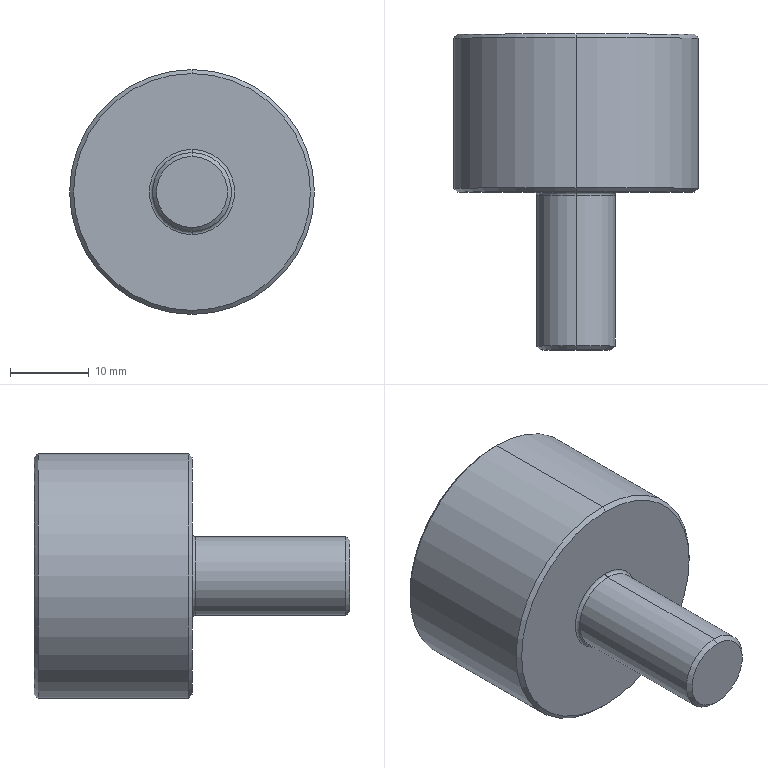Part | STEP file | OP10-133_seal rod camshaft | 1 solid | 25 faces | box 31 x 40 x 31 mm | volume 16299 mm3 | cylinder 10 | cone 8 | plane 5 | torus 2 | commonest cylinder face diameters 3.3 x2 6 x2 10 x2 11 x2 31 x2
STEP:
#1=CARTESIAN_POINT('',(0.,0.,0.));
#2=DIRECTION('',(0.,0.,1.));
#3=DIRECTION('',(1.,0.,0.));
#4=AXIS2_PLACEMENT_3D('',#1,#2,#3);
#5=CARTESIAN_POINT('',(0.,20.,5.4));
#6=VERTEX_POINT('',#5);
#7=CARTESIAN_POINT('',(0.,19.6,5.));
#8=VERTEX_POINT('',#7);
#9=CARTESIAN_POINT('',(0.,19.6,5.4));
#10=DIRECTION('',(-1.,0.,0.));
#11=DIRECTION('',(0.,0.,1.));
#12=AXIS2_PLACEMENT_3D('',#9,#10,#11);
#13=CIRCLE('',#12,0.4);
#14=CARTESIAN_POINT('',(0.,19.6,0.));
#15=DIRECTION('',(0.,1.,0.));
#16=DIRECTION('',(0.,0.,1.));
#17=AXIS2_PLACEMENT_3D('',#14,#15,#16);
#18=TOROIDAL_SURFACE('',#17,5.4,0.4);
#19=CARTESIAN_POINT('',(6.283,0.));
#20=DIRECTION('',(0.,1.));
#21=VECTOR('',#20,1.);
#22=LINE('',#19,#21);
#23=(GEOMETRIC_REPRESENTATION_CONTEXT(2)PARAMETRIC_REPRESENTATION_CONTEXT()REPRESENTATION_CONTEXT('',''));
#24=DEFINITIONAL_REPRESENTATION('',(#22),#23);
#25=PCURVE('',#18,#24);
#26=CARTESIAN_POINT('',(0.,19.6,0.));
#27=DIRECTION('',(0.,1.,0.));
#28=DIRECTION('',(0.,0.,1.));
#29=AXIS2_PLACEMENT_3D('',#26,#27,#28);
#30=TOROIDAL_SURFACE('',#29,5.4,0.4);
#31=CARTESIAN_POINT('',(0.,0.));
#32=DIRECTION('',(0.,1.));
#33=VECTOR('',#32,1.);
#34=LINE('',#31,#33);
#35=(GEOMETRIC_REPRESENTATION_CONTEXT(2)PARAMETRIC_REPRESENTATION_CONTEXT()REPRESENTATION_CONTEXT('',''));
#36=DEFINITIONAL_REPRESENTATION('',(#34),#35);
#37=PCURVE('',#30,#36);
#38=SURFACE_CURVE('',#13,(#25,#37),.PCURVE_S1.);
#39=EDGE_CURVE('',#6,#8,#38,.T.);
#40=ORIENTED_EDGE('',*,*,#39,.T.);
#41=CARTESIAN_POINT('',(0.,19.6,-5.));
#42=VERTEX_POINT('',#41);
#43=CARTESIAN_POINT('',(0.,19.6,0.));
#44=DIRECTION('',(0.,-1.,0.));
#45=DIRECTION('',(0.,0.,1.));
#46=AXIS2_PLACEMENT_3D('',#43,#44,#45);
#47=CIRCLE('',#46,5.);
#48=CARTESIAN_POINT('',(6.283,3.142));
#49=DIRECTION('',(-1.,0.));
#50=VECTOR('',#49,1.);
#51=LINE('',#48,#50);
#52=(GEOMETRIC_REPRESENTATION_CONTEXT(2)PARAMETRIC_REPRESENTATION_CONTEXT()REPRESENTATION_CONTEXT('',''));
#53=DEFINITIONAL_REPRESENTATION('',(#51),#52);
#54=PCURVE('',#18,#53);
#55=CARTESIAN_POINT('',(0.,20.,0.));
#56=DIRECTION('',(0.,-1.,0.));
#57=DIRECTION('',(0.,0.,-1.));
#58=AXIS2_PLACEMENT_3D('',#55,#56,#57);
#59=CYLINDRICAL_SURFACE('',#58,5.);
#60=CARTESIAN_POINT('',(3.142,0.4));
#61=DIRECTION('',(1.,0.));
#62=VECTOR('',#61,1.);
#63=LINE('',#60,#62);
#64=(GEOMETRIC_REPRESENTATION_CONTEXT(2)PARAMETRIC_REPRESENTATION_CONTEXT()REPRESENTATION_CONTEXT('',''));
#65=DEFINITIONAL_REPRESENTATION('',(#63),#64);
#66=PCURVE('',#59,#65);
#67=SURFACE_CURVE('',#47,(#54,#66),.PCURVE_S1.);
#68=EDGE_CURVE('',#8,#42,#67,.T.);
#69=ORIENTED_EDGE('',*,*,#68,.T.);
#70=CARTESIAN_POINT('',(0.,20.,-5.4));
#71=VERTEX_POINT('',#70);
#72=CARTESIAN_POINT('',(0.,19.6,-5.4));
#73=DIRECTION('',(1.,0.,0.));
#74=DIRECTION('',(0.,0.,-1.));
#75=AXIS2_PLACEMENT_3D('',#72,#73,#74);
#76=CIRCLE('',#75,0.4);
#77=CARTESIAN_POINT('',(3.142,0.));
#78=DIRECTION('',(0.,1.));
#79=VECTOR('',#78,1.);
#80=LINE('',#77,#79);
#81=(GEOMETRIC_REPRESENTATION_CONTEXT(2)PARAMETRIC_REPRESENTATION_CONTEXT()REPRESENTATION_CONTEXT('',''));
#82=DEFINITIONAL_REPRESENTATION('',(#80),#81);
#83=PCURVE('',#18,#82);
#84=CARTESIAN_POINT('',(3.142,0.));
#85=DIRECTION('',(0.,1.));
#86=VECTOR('',#85,1.);
#87=LINE('',#84,#86);
#88=(GEOMETRIC_REPRESENTATION_CONTEXT(2)PARAMETRIC_REPRESENTATION_CONTEXT()REPRESENTATION_CONTEXT('',''));
#89=DEFINITIONAL_REPRESENTATION('',(#87),#88);
#90=PCURVE('',#30,#89);
#91=SURFACE_CURVE('',#76,(#83,#90),.PCURVE_S1.);
#92=EDGE_CURVE('',#71,#42,#91,.T.);
#93=ORIENTED_EDGE('',*,*,#92,.F.);
#94=CARTESIAN_POINT('',(0.,20.,0.));
#95=DIRECTION('',(0.,1.,0.));
#96=DIRECTION('',(0.,0.,1.));
#97=AXIS2_PLACEMENT_3D('',#94,#95,#96);
#98=CIRCLE('',#97,5.4);
#99=CARTESIAN_POINT('',(0.,1.571));
#100=DIRECTION('',(1.,0.));
#101=VECTOR('',#100,1.);
#102=LINE('',#99,#101);
#103=(GEOMETRIC_REPRESENTATION_CONTEXT(2)PARAMETRIC_REPRESENTATION_CONTEXT()REPRESENTATION_CONTEXT('',''));
#104=DEFINITIONAL_REPRESENTATION('',(#102),#103);
#105=PCURVE('',#18,#104);
#106=CARTESIAN_POINT('',(0.,20.,0.));
#107=DIRECTION('',(0.,1.,0.));
#108=DIRECTION('',(0.,0.,1.));
#109=AXIS2_PLACEMENT_3D('',#106,#107,#108);
#110=PLANE('',#109);
#111=CARTESIAN_POINT('',(0.,0.));
#112=DIRECTION('',(1.,0.));
#113=AXIS2_PLACEMENT_2D('',#111,#112);
#114=CIRCLE('',#113,5.4);
#115=(GEOMETRIC_REPRESENTATION_CONTEXT(2)PARAMETRIC_REPRESENTATION_CONTEXT()REPRESENTATION_CONTEXT('',''));
#116=DEFINITIONAL_REPRESENTATION('',(#114),#115);
#117=PCURVE('',#110,#116);
#118=SURFACE_CURVE('',#98,(#105,#117),.PCURVE_S1.);
#119=EDGE_CURVE('',#71,#6,#118,.T.);
#120=ORIENTED_EDGE('',*,*,#119,.T.);
#121=EDGE_LOOP('',(#40,#69,#93,#120));
#122=FACE_BOUND('',#121,.F.);
#123=ADVANCED_FACE('',(#122),#18,.F.);
#124=CARTESIAN_POINT('',(0.,0.,-4.5));
#125=VERTEX_POINT('',#124);
#126=CARTESIAN_POINT('',(0.,0.,4.5));
#127=VERTEX_POINT('',#126);
#128=CARTESIAN_POINT('',(0.,0.,0.));
#129=DIRECTION('',(0.,-1.,0.));
#130=DIRECTION('',(0.,0.,1.));
#131=AXIS2_PLACEMENT_3D('',#128,#129,#130);
#132=CIRCLE('',#131,4.5);
#133=CARTESIAN_POINT('',(0.,0.5,0.));
#134=DIRECTION('',(0.,1.,0.));
#135=DIRECTION('',(0.,0.,1.));
#136=AXIS2_PLACEMENT_3D('',#133,#134,#135);
#137=CONICAL_SURFACE('',#136,5.,0.7854);
#138=CARTESIAN_POINT('',(6.283,-0.5));
#139=DIRECTION('',(-1.,0.));
#140=VECTOR('',#139,1.);
#141=LINE('',#138,#140);
#142=(GEOMETRIC_REPRESENTATION_CONTEXT(2)PARAMETRIC_REPRESENTATION_CONTEXT()REPRESENTATION_CONTEXT('',''));
#143=DEFINITIONAL_REPRESENTATION('',(#141),#142);
#144=PCURVE('',#137,#143);
#145=CARTESIAN_POINT('',(0.,0.,0.));
#146=DIRECTION('',(0.,1.,0.));
#147=DIRECTION('',(0.,0.,1.));
#148=AXIS2_PLACEMENT_3D('',#145,#146,#147);
#149=PLANE('',#148);
#150=CARTESIAN_POINT('',(4.5,0.));
#151=CARTESIAN_POINT('',(4.5,-7.794));
#152=CARTESIAN_POINT('',(-2.25,-3.897));
#153=CARTESIAN_POINT('',(-9.,0.));
#154=CARTESIAN_POINT('',(-2.25,3.897));
#155=CARTESIAN_POINT('',(4.5,7.794));
#156=CARTESIAN_POINT('',(4.5,0.));
#157=(BOUNDED_CURVE()B_SPLINE_CURVE(2,(#150,#151,#152,#153,#154,#155,#156),.UNSPECIFIED.,.T.,.F.)B_SPLINE_CURVE_WITH_KNOTS((1,2,2,2,2,1),(-2.094,0.,2.094,4.189,6.283,8.378),.UNSPECIFIED.)CURVE()GEOMETRIC_REPRESENTATION_ITEM()RATIONAL_B_SPLINE_CURVE((1.,0.5,1.,0.5,1.,0.5,1.))REPRESENTATION_ITEM(''));
#158=(GEOMETRIC_REPRESENTATION_CONTEXT(2)PARAMETRIC_REPRESENTATION_CONTEXT()REPRESENTATION_CONTEXT('',''));
#159=DEFINITIONAL_REPRESENTATION('',(#157),#158);
#160=PCURVE('',#149,#159);
#161=SURFACE_CURVE('',#132,(#144,#160),.PCURVE_S1.);
#162=EDGE_CURVE('',#125,#127,#161,.T.);
#163=ORIENTED_EDGE('',*,*,#162,.F.);
#164=CARTESIAN_POINT('',(0.,0.5,-5.));
#165=VERTEX_POINT('',#164);
#166=CARTESIAN_POINT('',(0.,0.5,-5.));
#167=DIRECTION('',(0.,0.7071,-0.7071));
#168=VECTOR('',#167,1.);
#169=LINE('',#166,#168);
#170=CARTESIAN_POINT('',(3.142,0.));
#171=DIRECTION('',(0.,1.));
#172=VECTOR('',#171,1.);
#173=LINE('',#170,#172);
#174=(GEOMETRIC_REPRESENTATION_CONTEXT(2)PARAMETRIC_REPRESENTATION_CONTEXT()REPRESENTATION_CONTEXT('',''));
#175=DEFINITIONAL_REPRESENTATION('',(#173),#174);
#176=PCURVE('',#137,#175);
#177=CARTESIAN_POINT('',(0.,0.5,0.));
#178=DIRECTION('',(0.,1.,0.));
#179=DIRECTION('',(0.,0.,1.));
#180=AXIS2_PLACEMENT_3D('',#177,#178,#179);
#181=CONICAL_SURFACE('',#180,5.,0.7854);
#182=CARTESIAN_POINT('',(3.142,0.));
#183=DIRECTION('',(0.,1.));
#184=VECTOR('',#183,1.);
#185=LINE('',#182,#184);
#186=(GEOMETRIC_REPRESENTATION_CONTEXT(2)PARAMETRIC_REPRESENTATION_CONTEXT()REPRESENTATION_CONTEXT('',''));
#187=DEFINITIONAL_REPRESENTATION('',(#185),#186);
#188=PCURVE('',#181,#187);
#189=SURFACE_CURVE('',#169,(#176,#188),.PCURVE_S1.);
#190=EDGE_CURVE('',#125,#165,#189,.T.);
#191=ORIENTED_EDGE('',*,*,#190,.T.);
#192=CARTESIAN_POINT('',(0.,0.5,5.));
#193=VERTEX_POINT('',#192);
#194=CARTESIAN_POINT('',(0.,0.5,0.));
#195=DIRECTION('',(0.,1.,0.));
#196=DIRECTION('',(0.,0.,1.));
#197=AXIS2_PLACEMENT_3D('',#194,#195,#196);
#198=CIRCLE('',#197,5.);
#199=CARTESIAN_POINT('',(0.,0.));
#200=DIRECTION('',(1.,0.));
#201=VECTOR('',#200,1.);
#202=LINE('',#199,#201);
#203=(GEOMETRIC_REPRESENTATION_CONTEXT(2)PARAMETRIC_REPRESENTATION_CONTEXT()REPRESENTATION_CONTEXT('',''));
#204=DEFINITIONAL_REPRESENTATION('',(#202),#203);
#205=PCURVE('',#137,#204);
#206=CARTESIAN_POINT('',(0.,20.,0.));
#207=DIRECTION('',(0.,-1.,0.));
#208=DIRECTION('',(0.,0.,-1.));
#209=AXIS2_PLACEMENT_3D('',#206,#207,#208);
#210=CYLINDRICAL_SURFACE('',#209,5.);
#211=CARTESIAN_POINT('',(3.142,19.5));
#212=DIRECTION('',(-1.,0.));
#213=VECTOR('',#212,1.);
#214=LINE('',#211,#213);
#215=(GEOMETRIC_REPRESENTATION_CONTEXT(2)PARAMETRIC_REPRESENTATION_CONTEXT()REPRESENTATION_CONTEXT('',''));
#216=DEFINITIONAL_REPRESENTATION('',(#214),#215);
#217=PCURVE('',#210,#216);
#218=SURFACE_CURVE('',#198,(#205,#217),.PCURVE_S1.);
#219=EDGE_CURVE('',#193,#165,#218,.T.);
#220=ORIENTED_EDGE('',*,*,#219,.F.);
#221=CARTESIAN_POINT('',(0.,0.5,5.));
#222=DIRECTION('',(0.,0.7071,0.7071));
#223=VECTOR('',#222,1.);
#224=LINE('',#221,#223);
#225=CARTESIAN_POINT('',(0.,0.));
#226=DIRECTION('',(0.,1.));
#227=VECTOR('',#226,1.);
#228=LINE('',#225,#227);
#229=(GEOMETRIC_REPRESENTATION_CONTEXT(2)PARAMETRIC_REPRESENTATION_CONTEXT()REPRESENTATION_CONTEXT('',''));
#230=DEFINITIONAL_REPRESENTATION('',(#228),#229);
#231=PCURVE('',#137,#230);
#232=CARTESIAN_POINT('',(6.283,0.));
#233=DIRECTION('',(0.,1.));
#234=VECTOR('',#233,1.);
#235=LINE('',#232,#234);
#236=(GEOMETRIC_REPRESENTATION_CONTEXT(2)PARAMETRIC_REPRESENTATION_CONTEXT()REPRESENTATION_CONTEXT('',''));
#237=DEFINITIONAL_REPRESENTATION('',(#235),#236);
#238=PCURVE('',#181,#237);
#239=SURFACE_CURVE('',#224,(#231,#238),.PCURVE_S1.);
#240=EDGE_CURVE('',#127,#193,#239,.T.);
#241=ORIENTED_EDGE('',*,*,#240,.F.);
#242=EDGE_LOOP('',(#163,#191,#220,#241));
#243=FACE_BOUND('',#242,.T.);
#244=ADVANCED_FACE('',(#243),#137,.T.);
#245=CARTESIAN_POINT('',(0.,40.,15.));
#246=VERTEX_POINT('',#245);
#247=CARTESIAN_POINT('',(0.,40.,-15.));
#248=VERTEX_POINT('',#247);
#249=CARTESIAN_POINT('',(0.,40.,0.));
#250=DIRECTION('',(0.,1.,0.));
#251=DIRECTION('',(0.,0.,1.));
#252=AXIS2_PLACEMENT_3D('',#249,#250,#251);
#253=CIRCLE('',#252,15.);
#254=CARTESIAN_POINT('',(0.,40.,0.));
#255=DIRECTION('',(0.,-1.,0.));
#256=DIRECTION('',(0.,0.,-1.));
#257=AXIS2_PLACEMENT_3D('',#254,#255,#256);
#258=CONICAL_SURFACE('',#257,15.,0.7854);
#259=CARTESIAN_POINT('',(3.142,0.));
#260=DIRECTION('',(-1.,0.));
#261=VECTOR('',#260,1.);
#262=LINE('',#259,#261);
#263=(GEOMETRIC_REPRESENTATION_CONTEXT(2)PARAMETRIC_REPRESENTATION_CONTEXT()REPRESENTATION_CONTEXT('',''));
#264=DEFINITIONAL_REPRESENTATION('',(#262),#263);
#265=PCURVE('',#258,#264);
#266=CARTESIAN_POINT('',(0.,40.,0.));
#267=DIRECTION('',(0.,1.,0.));
#268=DIRECTION('',(0.,0.,1.));
#269=AXIS2_PLACEMENT_3D('',#266,#267,#268);
#270=PLANE('',#269);
#271=CARTESIAN_POINT('',(0.,0.));
#272=DIRECTION('',(1.,0.));
#273=AXIS2_PLACEMENT_2D('',#271,#272);
#274=CIRCLE('',#273,15.);
#275=(GEOMETRIC_REPRESENTATION_CONTEXT(2)PARAMETRIC_REPRESENTATION_CONTEXT()REPRESENTATION_CONTEXT('',''));
#276=DEFINITIONAL_REPRESENTATION('',(#274),#275);
#277=PCURVE('',#270,#276);
#278=SURFACE_CURVE('',#253,(#265,#277),.PCURVE_S1.);
#279=EDGE_CURVE('',#246,#248,#278,.T.);
#280=ORIENTED_EDGE('',*,*,#279,.F.);
#281=CARTESIAN_POINT('',(0.,39.5,15.5));
#282=VERTEX_POINT('',#281);
#283=CARTESIAN_POINT('',(0.,40.,15.));
#284=DIRECTION('',(0.,-0.7071,0.7071));
#285=VECTOR('',#284,1.);
#286=LINE('',#283,#285);
#287=CARTESIAN_POINT('',(3.142,0.));
#288=DIRECTION('',(0.,1.));
#289=VECTOR('',#288,1.);
#290=LINE('',#287,#289);
#291=(GEOMETRIC_REPRESENTATION_CONTEXT(2)PARAMETRIC_REPRESENTATION_CONTEXT()REPRESENTATION_CONTEXT('',''));
#292=DEFINITIONAL_REPRESENTATION('',(#290),#291);
#293=PCURVE('',#258,#292);
#294=CARTESIAN_POINT('',(0.,40.,0.));
#295=DIRECTION('',(0.,-1.,0.));
#296=DIRECTION('',(0.,0.,-1.));
#297=AXIS2_PLACEMENT_3D('',#294,#295,#296);
#298=CONICAL_SURFACE('',#297,15.,0.7854);
#299=CARTESIAN_POINT('',(3.142,0.));
#300=DIRECTION('',(0.,1.));
#301=VECTOR('',#300,1.);
#302=LINE('',#299,#301);
#303=(GEOMETRIC_REPRESENTATION_CONTEXT(2)PARAMETRIC_REPRESENTATION_CONTEXT()REPRESENTATION_CONTEXT('',''));
#304=DEFINITIONAL_REPRESENTATION('',(#302),#303);
#305=PCURVE('',#298,#304);
#306=SURFACE_CURVE('',#286,(#293,#305),.PCURVE_S1.);
#307=EDGE_CURVE('',#246,#282,#306,.T.);
#308=ORIENTED_EDGE('',*,*,#307,.T.);
#309=CARTESIAN_POINT('',(0.,39.5,-15.5));
#310=VERTEX_POINT('',#309);
#311=CARTESIAN_POINT('',(0.,39.5,0.));
#312=DIRECTION('',(0.,-1.,0.));
#313=DIRECTION('',(0.,0.,1.));
#314=AXIS2_PLACEMENT_3D('',#311,#312,#313);
#315=CIRCLE('',#314,15.5);
#316=CARTESIAN_POINT('',(-3.142,0.5));
#317=DIRECTION('',(1.,0.));
#318=VECTOR('',#317,1.);
#319=LINE('',#316,#318);
#320=(GEOMETRIC_REPRESENTATION_CONTEXT(2)PARAMETRIC_REPRESENTATION_CONTEXT()REPRESENTATION_CONTEXT('',''));
#321=DEFINITIONAL_REPRESENTATION('',(#319),#320);
#322=PCURVE('',#258,#321);
#323=CARTESIAN_POINT('',(0.,40.,0.));
#324=DIRECTION('',(0.,-1.,0.));
#325=DIRECTION('',(0.,0.,-1.));
#326=AXIS2_PLACEMENT_3D('',#323,#324,#325);
#327=CYLINDRICAL_SURFACE('',#326,15.5);
#328=CARTESIAN_POINT('',(-3.142,0.5));
#329=DIRECTION('',(1.,0.));
#330=VECTOR('',#329,1.);
#331=LINE('',#328,#330);
#332=(GEOMETRIC_REPRESENTATION_CONTEXT(2)PARAMETRIC_REPRESENTATION_CONTEXT()REPRESENTATION_CONTEXT('',''));
#333=DEFINITIONAL_REPRESENTATION('',(#331),#332);
#334=PCURVE('',#327,#333);
#335=SURFACE_CURVE('',#315,(#322,#334),.PCURVE_S1.);
#336=EDGE_CURVE('',#310,#282,#335,.T.);
#337=ORIENTED_EDGE('',*,*,#336,.F.);
#338=CARTESIAN_POINT('',(0.,40.,-15.));
#339=DIRECTION('',(0.,-0.7071,-0.7071));
#340=VECTOR('',#339,1.);
#341=LINE('',#338,#340);
#342=CARTESIAN_POINT('',(0.,0.));
#343=DIRECTION('',(0.,1.));
#344=VECTOR('',#343,1.);
#345=LINE('',#342,#344);
#346=(GEOMETRIC_REPRESENTATION_CONTEXT(2)PARAMETRIC_REPRESENTATION_CONTEXT()REPRESENTATION_CONTEXT('',''));
#347=DEFINITIONAL_REPRESENTATION('',(#345),#346);
#348=PCURVE('',#258,#347);
#349=CARTESIAN_POINT('',(6.283,0.));
#350=DIRECTION('',(0.,1.));
#351=VECTOR('',#350,1.);
#352=LINE('',#349,#351);
#353=(GEOMETRIC_REPRESENTATION_CONTEXT(2)PARAMETRIC_REPRESENTATION_CONTEXT()REPRESENTATION_CONTEXT('',''));
#354=DEFINITIONAL_REPRESENTATION('',(#352),#353);
#355=PCURVE('',#298,#354);
#356=SURFACE_CURVE('',#341,(#348,#355),.PCURVE_S1.);
#357=EDGE_CURVE('',#248,#310,#356,.T.);
#358=ORIENTED_EDGE('',*,*,#357,.F.);
#359=EDGE_LOOP('',(#280,#308,#337,#358));
#360=FACE_BOUND('',#359,.T.);
#361=ADVANCED_FACE('',(#360),#258,.T.);
#362=CARTESIAN_POINT('',(0.,20.,-15.));
#363=VERTEX_POINT('',#362);
#364=CARTESIAN_POINT('',(0.,20.,15.));
#365=VERTEX_POINT('',#364);
#366=CARTESIAN_POINT('',(0.,20.,0.));
#367=DIRECTION('',(0.,-1.,0.));
#368=DIRECTION('',(0.,0.,1.));
#369=AXIS2_PLACEMENT_3D('',#366,#367,#368);
#370=CIRCLE('',#369,15.);
#371=CARTESIAN_POINT('',(0.,20.5,0.));
#372=DIRECTION('',(0.,1.,0.));
#373=DIRECTION('',(0.,0.,1.));
#374=AXIS2_PLACEMENT_3D('',#371,#372,#373);
#375=CONICAL_SURFACE('',#374,15.5,0.7854);
#376=CARTESIAN_POINT('',(6.283,-0.5));
#377=DIRECTION('',(-1.,0.));
#378=VECTOR('',#377,1.);
#379=LINE('',#376,#378);
#380=(GEOMETRIC_REPRESENTATION_CONTEXT(2)PARAMETRIC_REPRESENTATION_CONTEXT()REPRESENTATION_CONTEXT('',''));
#381=DEFINITIONAL_REPRESENTATION('',(#379),#380);
#382=PCURVE('',#375,#381);
#383=CARTESIAN_POINT('',(15.,0.));
#384=CARTESIAN_POINT('',(15.,-25.981));
#385=CARTESIAN_POINT('',(-7.5,-12.99));
#386=CARTESIAN_POINT('',(-30.,0.));
#387=CARTESIAN_POINT('',(-7.5,12.99));
#388=CARTESIAN_POINT('',(15.,25.981));
#389=CARTESIAN_POINT('',(15.,0.));
#390=(BOUNDED_CURVE()B_SPLINE_CURVE(2,(#383,#384,#385,#386,#387,#388,#389),.UNSPECIFIED.,.T.,.F.)B_SPLINE_CURVE_WITH_KNOTS((1,2,2,2,2,1),(-2.094,0.,2.094,4.189,6.283,8.378),.UNSPECIFIED.)CURVE()GEOMETRIC_REPRESENTATION_ITEM()RATIONAL_B_SPLINE_CURVE((1.,0.5,1.,0.5,1.,0.5,1.))REPRESENTATION_ITEM(''));
#391=(GEOMETRIC_REPRESENTATION_CONTEXT(2)PARAMETRIC_REPRESENTATION_CONTEXT()REPRESENTATION_CONTEXT('',''));
#392=DEFINITIONAL_REPRESENTATION('',(#390),#391);
#393=PCURVE('',#110,#392);
#394=SURFACE_CURVE('',#370,(#382,#393),.PCURVE_S1.);
#395=EDGE_CURVE('',#363,#365,#394,.T.);
#396=ORIENTED_EDGE('',*,*,#395,.F.);
#397=CARTESIAN_POINT('',(0.,20.5,-15.5));
#398=VERTEX_POINT('',#397);
#399=CARTESIAN_POINT('',(0.,20.5,-15.5));
#400=DIRECTION('',(0.,0.7071,-0.7071));
#401=VECTOR('',#400,1.);
#402=LINE('',#399,#401);
#403=CARTESIAN_POINT('',(3.142,0.));
#404=DIRECTION('',(0.,1.));
#405=VECTOR('',#404,1.);
#406=LINE('',#403,#405);
#407=(GEOMETRIC_REPRESENTATION_CONTEXT(2)PARAMETRIC_REPRESENTATION_CONTEXT()REPRESENTATION_CONTEXT('',''));
#408=DEFINITIONAL_REPRESENTATION('',(#406),#407);
#409=PCURVE('',#375,#408);
#410=CARTESIAN_POINT('',(0.,20.5,0.));
#411=DIRECTION('',(0.,1.,0.));
#412=DIRECTION('',(0.,0.,1.));
#413=AXIS2_PLACEMENT_3D('',#410,#411,#412);
#414=CONICAL_SURFACE('',#413,15.5,0.7854);
#415=CARTESIAN_POINT('',(3.142,0.));
#416=DIRECTION('',(0.,1.));
#417=VECTOR('',#416,1.);
#418=LINE('',#415,#417);
#419=(GEOMETRIC_REPRESENTATION_CONTEXT(2)PARAMETRIC_REPRESENTATION_CONTEXT()REPRESENTATION_CONTEXT('',''));
#420=DEFINITIONAL_REPRESENTATION('',(#418),#419);
#421=PCURVE('',#414,#420);
#422=SURFACE_CURVE('',#402,(#409,#421),.PCURVE_S1.);
#423=EDGE_CURVE('',#363,#398,#422,.T.);
#424=ORIENTED_EDGE('',*,*,#423,.T.);
#425=CARTESIAN_POINT('',(0.,20.5,15.5));
#426=VERTEX_POINT('',#425);
#427=CARTESIAN_POINT('',(0.,20.5,0.));
#428=DIRECTION('',(0.,1.,0.));
#429=DIRECTION('',(0.,0.,1.));
#430=AXIS2_PLACEMENT_3D('',#427,#428,#429);
#431=CIRCLE('',#430,15.5);
#432=CARTESIAN_POINT('',(0.,0.));
#433=DIRECTION('',(1.,0.));
#434=VECTOR('',#433,1.);
#435=LINE('',#432,#434);
#436=(GEOMETRIC_REPRESENTATION_CONTEXT(2)PARAMETRIC_REPRESENTATION_CONTEXT()REPRESENTATION_CONTEXT('',''));
#437=DEFINITIONAL_REPRESENTATION('',(#435),#436);
#438=PCURVE('',#375,#437);
#439=CARTESIAN_POINT('',(3.142,19.5));
#440=DIRECTION('',(-1.,0.));
#441=VECTOR('',#440,1.);
#442=LINE('',#439,#441);
#443=(GEOMETRIC_REPRESENTATION_CONTEXT(2)PARAMETRIC_REPRESENTATION_CONTEXT()REPRESENTATION_CONTEXT('',''));
#444=DEFINITIONAL_REPRESENTATION('',(#442),#443);
#445=PCURVE('',#327,#444);
#446=SURFACE_CURVE('',#431,(#438,#445),.PCURVE_S1.);
#447=EDGE_CURVE('',#426,#398,#446,.T.);
#448=ORIENTED_EDGE('',*,*,#447,.F.);
#449=CARTESIAN_POINT('',(0.,20.5,15.5));
#450=DIRECTION('',(0.,0.7071,0.7071));
#451=VECTOR('',#450,1.);
#452=LINE('',#449,#451);
#453=CARTESIAN_POINT('',(0.,0.));
#454=DIRECTION('',(0.,1.));
#455=VECTOR('',#454,1.);
#456=LINE('',#453,#455);
#457=(GEOMETRIC_REPRESENTATION_CONTEXT(2)PARAMETRIC_REPRESENTATION_CONTEXT()REPRESENTATION_CONTEXT('',''));
#458=DEFINITIONAL_REPRESENTATION('',(#456),#457);
#459=PCURVE('',#375,#458);
#460=CARTESIAN_POINT('',(6.283,0.));
#461=DIRECTION('',(0.,1.));
#462=VECTOR('',#461,1.);
#463=LINE('',#460,#462);
#464=(GEOMETRIC_REPRESENTATION_CONTEXT(2)PARAMETRIC_REPRESENTATION_CONTEXT()REPRESENTATION_CONTEXT('',''));
#465=DEFINITIONAL_REPRESENTATION('',(#463),#464);
#466=PCURVE('',#414,#465);
#467=SURFACE_CURVE('',#452,(#459,#466),.PCURVE_S1.);
#468=EDGE_CURVE('',#365,#426,#467,.T.);
#469=ORIENTED_EDGE('',*,*,#468,.F.);
#470=EDGE_LOOP('',(#396,#424,#448,#469));
#471=FACE_BOUND('',#470,.T.);
#472=ADVANCED_FACE('',(#471),#375,.T.);
#473=CARTESIAN_POINT('',(0.,23.,1.65));
#474=VERTEX_POINT('',#473);
#475=CARTESIAN_POINT('',(0.,35.,1.65));
#476=VERTEX_POINT('',#475);
#477=CARTESIAN_POINT('',(0.,35.,1.65));
#478=DIRECTION('',(0.,1.,0.));
#479=VECTOR('',#478,1.);
#480=LINE('',#477,#479);
#481=CARTESIAN_POINT('',(0.,35.,0.));
#482=DIRECTION('',(0.,1.,0.));
#483=DIRECTION('',(0.,0.,1.));
#484=AXIS2_PLACEMENT_3D('',#481,#482,#483);
#485=CYLINDRICAL_SURFACE('',#484,1.65);
#486=CARTESIAN_POINT('',(6.283,0.));
#487=DIRECTION('',(0.,1.));
#488=VECTOR('',#487,1.);
#489=LINE('',#486,#488);
#490=(GEOMETRIC_REPRESENTATION_CONTEXT(2)PARAMETRIC_REPRESENTATION_CONTEXT()REPRESENTATION_CONTEXT('',''));
#491=DEFINITIONAL_REPRESENTATION('',(#489),#490);
#492=PCURVE('',#485,#491);
#493=CARTESIAN_POINT('',(0.,35.,0.));
#494=DIRECTION('',(0.,1.,0.));
#495=DIRECTION('',(0.,0.,1.));
#496=AXIS2_PLACEMENT_3D('',#493,#494,#495);
#497=CYLINDRICAL_SURFACE('',#496,1.65);
#498=CARTESIAN_POINT('',(0.,0.));
#499=DIRECTION('',(0.,1.));
#500=VECTOR('',#499,1.);
#501=LINE('',#498,#500);
#502=(GEOMETRIC_REPRESENTATION_CONTEXT(2)PARAMETRIC_REPRESENTATION_CONTEXT()REPRESENTATION_CONTEXT('',''));
#503=DEFINITIONAL_REPRESENTATION('',(#501),#502);
#504=PCURVE('',#497,#503);
#505=SURFACE_CURVE('',#480,(#492,#504),.PCURVE_S1.);
#506=EDGE_CURVE('',#474,#476,#505,.T.);
#507=ORIENTED_EDGE('',*,*,#506,.T.);
#508=CARTESIAN_POINT('',(0.,35.,-1.65));
#509=VERTEX_POINT('',#508);
#510=CARTESIAN_POINT('',(0.,35.,0.));
#511=DIRECTION('',(0.,1.,0.));
#512=DIRECTION('',(0.,0.,1.));
#513=AXIS2_PLACEMENT_3D('',#510,#511,#512);
#514=CIRCLE('',#513,1.65);
#515=CARTESIAN_POINT('',(0.,0.));
#516=DIRECTION('',(1.,0.));
#517=VECTOR('',#516,1.);
#518=LINE('',#515,#517);
#519=(GEOMETRIC_REPRESENTATION_CONTEXT(2)PARAMETRIC_REPRESENTATION_CONTEXT()REPRESENTATION_CONTEXT('',''));
#520=DEFINITIONAL_REPRESENTATION('',(#518),#519);
#521=PCURVE('',#485,#520);
#522=CARTESIAN_POINT('',(0.,35.,0.));
#523=DIRECTION('',(0.,1.,0.));
#524=DIRECTION('',(0.,0.,1.));
#525=AXIS2_PLACEMENT_3D('',#522,#523,#524);
#526=PLANE('',#525);
#527=CARTESIAN_POINT('',(0.,0.));
#528=DIRECTION('',(1.,0.));
#529=AXIS2_PLACEMENT_2D('',#527,#528);
#530=CIRCLE('',#529,1.65);
#531=(GEOMETRIC_REPRESENTATION_CONTEXT(2)PARAMETRIC_REPRESENTATION_CONTEXT()REPRESENTATION_CONTEXT('',''));
#532=DEFINITIONAL_REPRESENTATION('',(#530),#531);
#533=PCURVE('',#526,#532);
#534=SURFACE_CURVE('',#514,(#521,#533),.PCURVE_S1.);
#535=EDGE_CURVE('',#509,#476,#534,.T.);
#536=ORIENTED_EDGE('',*,*,#535,.F.);
#537=CARTESIAN_POINT('',(0.,23.,-1.65));
#538=VERTEX_POINT('',#537);
#539=CARTESIAN_POINT('',(0.,35.,-1.65));
#540=DIRECTION('',(0.,1.,0.));
#541=VECTOR('',#540,1.);
#542=LINE('',#539,#541);
#543=CARTESIAN_POINT('',(3.142,0.));
#544=DIRECTION('',(0.,1.));
#545=VECTOR('',#544,1.);
#546=LINE('',#543,#545);
#547=(GEOMETRIC_REPRESENTATION_CONTEXT(2)PARAMETRIC_REPRESENTATION_CONTEXT()REPRESENTATION_CONTEXT('',''));
#548=DEFINITIONAL_REPRESENTATION('',(#546),#547);
#549=PCURVE('',#485,#548);
#550=CARTESIAN_POINT('',(3.142,0.));
#551=DIRECTION('',(0.,1.));
#552=VECTOR('',#551,1.);
#553=LINE('',#550,#552);
#554=(GEOMETRIC_REPRESENTATION_CONTEXT(2)PARAMETRIC_REPRESENTATION_CONTEXT()REPRESENTATION_CONTEXT('',''));
#555=DEFINITIONAL_REPRESENTATION('',(#553),#554);
#556=PCURVE('',#497,#555);
#557=SURFACE_CURVE('',#542,(#549,#556),.PCURVE_S1.);
#558=EDGE_CURVE('',#538,#509,#557,.T.);
#559=ORIENTED_EDGE('',*,*,#558,.F.);
#560=CARTESIAN_POINT('',(0.,23.,0.));
#561=DIRECTION('',(0.,1.,0.));
#562=DIRECTION('',(0.,0.,1.));
#563=AXIS2_PLACEMENT_3D('',#560,#561,#562);
#564=CIRCLE('',#563,1.65);
#565=CARTESIAN_POINT('',(0.,-12.));
#566=DIRECTION('',(1.,0.));
#567=VECTOR('',#566,1.);
#568=LINE('',#565,#567);
#569=(GEOMETRIC_REPRESENTATION_CONTEXT(2)PARAMETRIC_REPRESENTATION_CONTEXT()REPRESENTATION_CONTEXT('',''));
#570=DEFINITIONAL_REPRESENTATION('',(#568),#569);
#571=PCURVE('',#485,#570);
#572=CARTESIAN_POINT('',(0.,23.,0.));
#573=DIRECTION('',(0.,1.,0.));
#574=DIRECTION('',(0.,0.,1.));
#575=AXIS2_PLACEMENT_3D('',#572,#573,#574);
#576=CONICAL_SURFACE('',#575,1.65,1.03);
#577=CARTESIAN_POINT('',(0.,0.));
#578=DIRECTION('',(1.,0.));
#579=VECTOR('',#578,1.);
#580=LINE('',#577,#579);
#581=(GEOMETRIC_REPRESENTATION_CONTEXT(2)PARAMETRIC_REPRESENTATION_CONTEXT()REPRESENTATION_CONTEXT('',''));
#582=DEFINITIONAL_REPRESENTATION('',(#580),#581);
#583=PCURVE('',#576,#582);
#584=SURFACE_CURVE('',#564,(#571,#583),.PCURVE_S1.);
#585=EDGE_CURVE('',#538,#474,#584,.T.);
#586=ORIENTED_EDGE('',*,*,#585,.T.);
#587=EDGE_LOOP('',(#507,#536,#559,#586));
#588=FACE_BOUND('',#587,.F.);
#589=ADVANCED_FACE('',(#588),#485,.F.);
#590=ORIENTED_EDGE('',*,*,#585,.F.);
#591=CARTESIAN_POINT('',(0.,22.009,0.));
#592=VERTEX_POINT('',#591);
#593=CARTESIAN_POINT('',(0.,23.,-1.65));
#594=DIRECTION('',(0.,0.515,-0.8572));
#595=VECTOR('',#594,1.);
#596=LINE('',#593,#595);
#597=CARTESIAN_POINT('',(3.142,0.));
#598=DIRECTION('',(0.,1.));
#599=VECTOR('',#598,1.);
#600=LINE('',#597,#599);
#601=(GEOMETRIC_REPRESENTATION_CONTEXT(2)PARAMETRIC_REPRESENTATION_CONTEXT()REPRESENTATION_CONTEXT('',''));
#602=DEFINITIONAL_REPRESENTATION('',(#600),#601);
#603=PCURVE('',#576,#602);
#604=CARTESIAN_POINT('',(0.,23.,0.));
#605=DIRECTION('',(0.,1.,0.));
#606=DIRECTION('',(0.,0.,1.));
#607=AXIS2_PLACEMENT_3D('',#604,#605,#606);
#608=CONICAL_SURFACE('',#607,1.65,1.03);
#609=CARTESIAN_POINT('',(3.142,0.));
#610=DIRECTION('',(0.,1.));
#611=VECTOR('',#610,1.);
#612=LINE('',#609,#611);
#613=(GEOMETRIC_REPRESENTATION_CONTEXT(2)PARAMETRIC_REPRESENTATION_CONTEXT()REPRESENTATION_CONTEXT('',''));
#614=DEFINITIONAL_REPRESENTATION('',(#612),#613);
#615=PCURVE('',#608,#614);
#616=SURFACE_CURVE('',#596,(#603,#615),.PCURVE_S1.);
#617=EDGE_CURVE('',#592,#538,#616,.T.);
#618=ORIENTED_EDGE('',*,*,#617,.F.);
#619=CARTESIAN_POINT('',(0.,23.,1.65));
#620=DIRECTION('',(0.,0.515,0.8572));
#621=VECTOR('',#620,1.);
#622=LINE('',#619,#621);
#623=CARTESIAN_POINT('',(6.283,0.));
#624=DIRECTION('',(0.,1.));
#625=VECTOR('',#624,1.);
#626=LINE('',#623,#625);
#627=(GEOMETRIC_REPRESENTATION_CONTEXT(2)PARAMETRIC_REPRESENTATION_CONTEXT()REPRESENTATION_CONTEXT('',''));
#628=DEFINITIONAL_REPRESENTATION('',(#626),#627);
#629=PCURVE('',#576,#628);
#630=CARTESIAN_POINT('',(0.,0.));
#631=DIRECTION('',(0.,1.));
#632=VECTOR('',#631,1.);
#633=LINE('',#630,#632);
#634=(GEOMETRIC_REPRESENTATION_CONTEXT(2)PARAMETRIC_REPRESENTATION_CONTEXT()REPRESENTATION_CONTEXT('',''));
#635=DEFINITIONAL_REPRESENTATION('',(#633),#634);
#636=PCURVE('',#608,#635);
#637=SURFACE_CURVE('',#622,(#629,#636),.PCURVE_S1.);
#638=EDGE_CURVE('',#592,#474,#637,.T.);
#639=ORIENTED_EDGE('',*,*,#638,.T.);
#640=EDGE_LOOP('',(#590,#618,#639));
#641=FACE_BOUND('',#640,.F.);
#642=ADVANCED_FACE('',(#641),#576,.F.);
#643=CARTESIAN_POINT('',(0.,35.,3.));
#644=VERTEX_POINT('',#643);
#645=CARTESIAN_POINT('',(0.,38.6,3.));
#646=VERTEX_POINT('',#645);
#647=CARTESIAN_POINT('',(0.,35.,3.));
#648=DIRECTION('',(0.,1.,0.));
#649=VECTOR('',#648,1.);
#650=LINE('',#647,#649);
#651=CARTESIAN_POINT('',(0.,35.,0.));
#652=DIRECTION('',(0.,1.,0.));
#653=DIRECTION('',(0.,0.,1.));
#654=AXIS2_PLACEMENT_3D('',#651,#652,#653);
#655=CYLINDRICAL_SURFACE('',#654,3.);
#656=CARTESIAN_POINT('',(6.283,0.));
#657=DIRECTION('',(0.,1.));
#658=VECTOR('',#657,1.);
#659=LINE('',#656,#658);
#660=(GEOMETRIC_REPRESENTATION_CONTEXT(2)PARAMETRIC_REPRESENTATION_CONTEXT()REPRESENTATION_CONTEXT('',''));
#661=DEFINITIONAL_REPRESENTATION('',(#659),#660);
#662=PCURVE('',#655,#661);
#663=CARTESIAN_POINT('',(0.,35.,0.));
#664=DIRECTION('',(0.,1.,0.));
#665=DIRECTION('',(0.,0.,1.));
#666=AXIS2_PLACEMENT_3D('',#663,#664,#665);
#667=CYLINDRICAL_SURFACE('',#666,3.);
#668=CARTESIAN_POINT('',(0.,0.));
#669=DIRECTION('',(0.,1.));
#670=VECTOR('',#669,1.);
#671=LINE('',#668,#670);
#672=(GEOMETRIC_REPRESENTATION_CONTEXT(2)PARAMETRIC_REPRESENTATION_CONTEXT()REPRESENTATION_CONTEXT('',''));
#673=DEFINITIONAL_REPRESENTATION('',(#671),#672);
#674=PCURVE('',#667,#673);
#675=SURFACE_CURVE('',#650,(#662,#674),.PCURVE_S1.);
#676=EDGE_CURVE('',#644,#646,#675,.T.);
#677=ORIENTED_EDGE('',*,*,#676,.T.);
#678=CARTESIAN_POINT('',(0.,38.6,-3.));
#679=VERTEX_POINT('',#678);
#680=CARTESIAN_POINT('',(0.,38.6,0.));
#681=DIRECTION('',(0.,1.,0.));
#682=DIRECTION('',(0.,0.,1.));
#683=AXIS2_PLACEMENT_3D('',#680,#681,#682);
#684=CIRCLE('',#683,3.);
#685=CARTESIAN_POINT('',(0.,3.6));
#686=DIRECTION('',(1.,0.));
#687=VECTOR('',#686,1.);
#688=LINE('',#685,#687);
#689=(GEOMETRIC_REPRESENTATION_CONTEXT(2)PARAMETRIC_REPRESENTATION_CONTEXT()REPRESENTATION_CONTEXT('',''));
#690=DEFINITIONAL_REPRESENTATION('',(#688),#689);
#691=PCURVE('',#655,#690);
#692=CARTESIAN_POINT('',(0.,38.6,0.));
#693=DIRECTION('',(0.,1.,0.));
#694=DIRECTION('',(0.,0.,1.));
#695=AXIS2_PLACEMENT_3D('',#692,#693,#694);
#696=PLANE('',#695);
#697=CARTESIAN_POINT('',(0.,0.));
#698=DIRECTION('',(1.,0.));
#699=AXIS2_PLACEMENT_2D('',#697,#698);
#700=CIRCLE('',#699,3.);
#701=(GEOMETRIC_REPRESENTATION_CONTEXT(2)PARAMETRIC_REPRESENTATION_CONTEXT()REPRESENTATION_CONTEXT('',''));
#702=DEFINITIONAL_REPRESENTATION('',(#700),#701);
#703=PCURVE('',#696,#702);
#704=SURFACE_CURVE('',#684,(#691,#703),.PCURVE_S1.);
#705=EDGE_CURVE('',#679,#646,#704,.T.);
#706=ORIENTED_EDGE('',*,*,#705,.F.);
#707=CARTESIAN_POINT('',(0.,35.,-3.));
#708=VERTEX_POINT('',#707);
#709=CARTESIAN_POINT('',(0.,35.,-3.));
#710=DIRECTION('',(0.,1.,0.));
#711=VECTOR('',#710,1.);
#712=LINE('',#709,#711);
#713=CARTESIAN_POINT('',(3.142,0.));
#714=DIRECTION('',(0.,1.));
#715=VECTOR('',#714,1.);
#716=LINE('',#713,#715);
#717=(GEOMETRIC_REPRESENTATION_CONTEXT(2)PARAMETRIC_REPRESENTATION_CONTEXT()REPRESENTATION_CONTEXT('',''));
#718=DEFINITIONAL_REPRESENTATION('',(#716),#717);
#719=PCURVE('',#655,#718);
#720=CARTESIAN_POINT('',(3.142,0.));
#721=DIRECTION('',(0.,1.));
#722=VECTOR('',#721,1.);
#723=LINE('',#720,#722);
#724=(GEOMETRIC_REPRESENTATION_CONTEXT(2)PARAMETRIC_REPRESENTATION_CONTEXT()REPRESENTATION_CONTEXT('',''));
#725=DEFINITIONAL_REPRESENTATION('',(#723),#724);
#726=PCURVE('',#667,#725);
#727=SURFACE_CURVE('',#712,(#719,#726),.PCURVE_S1.);
#728=EDGE_CURVE('',#708,#679,#727,.T.);
#729=ORIENTED_EDGE('',*,*,#728,.F.);
#730=CARTESIAN_POINT('',(0.,35.,0.));
#731=DIRECTION('',(0.,1.,0.));
#732=DIRECTION('',(0.,0.,1.));
#733=AXIS2_PLACEMENT_3D('',#730,#731,#732);
#734=CIRCLE('',#733,3.);
#735=CARTESIAN_POINT('',(0.,0.));
#736=DIRECTION('',(1.,0.));
#737=VECTOR('',#736,1.);
#738=LINE('',#735,#737);
#739=(GEOMETRIC_REPRESENTATION_CONTEXT(2)PARAMETRIC_REPRESENTATION_CONTEXT()REPRESENTATION_CONTEXT('',''));
#740=DEFINITIONAL_REPRESENTATION('',(#738),#739);
#741=PCURVE('',#655,#740);
#742=CARTESIAN_POINT('',(0.,0.));
#743=DIRECTION('',(1.,0.));
#744=AXIS2_PLACEMENT_2D('',#742,#743);
#745=CIRCLE('',#744,3.);
#746=(GEOMETRIC_REPRESENTATION_CONTEXT(2)PARAMETRIC_REPRESENTATION_CONTEXT()REPRESENTATION_CONTEXT('',''));
#747=DEFINITIONAL_REPRESENTATION('',(#745),#746);
#748=PCURVE('',#526,#747);
#749=SURFACE_CURVE('',#734,(#741,#748),.PCURVE_S1.);
#750=EDGE_CURVE('',#708,#644,#749,.T.);
#751=ORIENTED_EDGE('',*,*,#750,.T.);
#752=EDGE_LOOP('',(#677,#706,#729,#751));
#753=FACE_BOUND('',#752,.F.);
#754=ADVANCED_FACE('',(#753),#655,.F.);
#755=CARTESIAN_POINT('',(0.,38.6,5.5));
#756=VERTEX_POINT('',#755);
#757=CARTESIAN_POINT('',(0.,40.,5.5));
#758=VERTEX_POINT('',#757);
#759=CARTESIAN_POINT('',(0.,38.6,5.5));
#760=DIRECTION('',(0.,1.,0.));
#761=VECTOR('',#760,1.);
#762=LINE('',#759,#761);
#763=CARTESIAN_POINT('',(0.,38.6,0.));
#764=DIRECTION('',(0.,1.,0.));
#765=DIRECTION('',(0.,0.,1.));
#766=AXIS2_PLACEMENT_3D('',#763,#764,#765);
#767=CYLINDRICAL_SURFACE('',#766,5.5);
#768=CARTESIAN_POINT('',(6.283,0.));
#769=DIRECTION('',(0.,1.));
#770=VECTOR('',#769,1.);
#771=LINE('',#768,#770);
#772=(GEOMETRIC_REPRESENTATION_CONTEXT(2)PARAMETRIC_REPRESENTATION_CONTEXT()REPRESENTATION_CONTEXT('',''));
#773=DEFINITIONAL_REPRESENTATION('',(#771),#772);
#774=PCURVE('',#767,#773);
#775=CARTESIAN_POINT('',(0.,38.6,0.));
#776=DIRECTION('',(0.,1.,0.));
#777=DIRECTION('',(0.,0.,1.));
#778=AXIS2_PLACEMENT_3D('',#775,#776,#777);
#779=CYLINDRICAL_SURFACE('',#778,5.5);
#780=CARTESIAN_POINT('',(0.,0.));
#781=DIRECTION('',(0.,1.));
#782=VECTOR('',#781,1.);
#783=LINE('',#780,#782);
#784=(GEOMETRIC_REPRESENTATION_CONTEXT(2)PARAMETRIC_REPRESENTATION_CONTEXT()REPRESENTATION_CONTEXT('',''));
#785=DEFINITIONAL_REPRESENTATION('',(#783),#784);
#786=PCURVE('',#779,#785);
#787=SURFACE_CURVE('',#762,(#774,#786),.PCURVE_S1.);
#788=EDGE_CURVE('',#756,#758,#787,.T.);
#789=ORIENTED_EDGE('',*,*,#788,.T.);
#790=CARTESIAN_POINT('',(0.,40.,-5.5));
#791=VERTEX_POINT('',#790);
#792=CARTESIAN_POINT('',(0.,40.,0.));
#793=DIRECTION('',(0.,1.,0.));
#794=DIRECTION('',(0.,0.,1.));
#795=AXIS2_PLACEMENT_3D('',#792,#793,#794);
#796=CIRCLE('',#795,5.5);
#797=CARTESIAN_POINT('',(0.,1.4));
#798=DIRECTION('',(1.,0.));
#799=VECTOR('',#798,1.);
#800=LINE('',#797,#799);
#801=(GEOMETRIC_REPRESENTATION_CONTEXT(2)PARAMETRIC_REPRESENTATION_CONTEXT()REPRESENTATION_CONTEXT('',''));
#802=DEFINITIONAL_REPRESENTATION('',(#800),#801);
#803=PCURVE('',#767,#802);
#804=CARTESIAN_POINT('',(0.,0.));
#805=DIRECTION('',(1.,0.));
#806=AXIS2_PLACEMENT_2D('',#804,#805);
#807=CIRCLE('',#806,5.5);
#808=(GEOMETRIC_REPRESENTATION_CONTEXT(2)PARAMETRIC_REPRESENTATION_CONTEXT()REPRESENTATION_CONTEXT('',''));
#809=DEFINITIONAL_REPRESENTATION('',(#807),#808);
#810=PCURVE('',#270,#809);
#811=SURFACE_CURVE('',#796,(#803,#810),.PCURVE_S1.);
#812=EDGE_CURVE('',#791,#758,#811,.T.);
#813=ORIENTED_EDGE('',*,*,#812,.F.);
#814=CARTESIAN_POINT('',(0.,38.6,-5.5));
#815=VERTEX_POINT('',#814);
#816=CARTESIAN_POINT('',(0.,38.6,-5.5));
#817=DIRECTION('',(0.,1.,0.));
#818=VECTOR('',#817,1.);
#819=LINE('',#816,#818);
#820=CARTESIAN_POINT('',(3.142,0.));
#821=DIRECTION('',(0.,1.));
#822=VECTOR('',#821,1.);
#823=LINE('',#820,#822);
#824=(GEOMETRIC_REPRESENTATION_CONTEXT(2)PARAMETRIC_REPRESENTATION_CONTEXT()REPRESENTATION_CONTEXT('',''));
#825=DEFINITIONAL_REPRESENTATION('',(#823),#824);
#826=PCURVE('',#767,#825);
#827=CARTESIAN_POINT('',(3.142,0.));
#828=DIRECTION('',(0.,1.));
#829=VECTOR('',#828,1.);
#830=LINE('',#827,#829);
#831=(GEOMETRIC_REPRESENTATION_CONTEXT(2)PARAMETRIC_REPRESENTATION_CONTEXT()REPRESENTATION_CONTEXT('',''));
#832=DEFINITIONAL_REPRESENTATION('',(#830),#831);
#833=PCURVE('',#779,#832);
#834=SURFACE_CURVE('',#819,(#826,#833),.PCURVE_S1.);
#835=EDGE_CURVE('',#815,#791,#834,.T.);
#836=ORIENTED_EDGE('',*,*,#835,.F.);
#837=CARTESIAN_POINT('',(0.,38.6,0.));
#838=DIRECTION('',(0.,1.,0.));
#839=DIRECTION('',(0.,0.,1.));
#840=AXIS2_PLACEMENT_3D('',#837,#838,#839);
#841=CIRCLE('',#840,5.5);
#842=CARTESIAN_POINT('',(0.,0.));
#843=DIRECTION('',(1.,0.));
#844=VECTOR('',#843,1.);
#845=LINE('',#842,#844);
#846=(GEOMETRIC_REPRESENTATION_CONTEXT(2)PARAMETRIC_REPRESENTATION_CONTEXT()REPRESENTATION_CONTEXT('',''));
#847=DEFINITIONAL_REPRESENTATION('',(#845),#846);
#848=PCURVE('',#767,#847);
#849=CARTESIAN_POINT('',(0.,0.));
#850=DIRECTION('',(1.,0.));
#851=AXIS2_PLACEMENT_2D('',#849,#850);
#852=CIRCLE('',#851,5.5);
#853=(GEOMETRIC_REPRESENTATION_CONTEXT(2)PARAMETRIC_REPRESENTATION_CONTEXT()REPRESENTATION_CONTEXT('',''));
#854=DEFINITIONAL_REPRESENTATION('',(#852),#853);
#855=PCURVE('',#696,#854);
#856=SURFACE_CURVE('',#841,(#848,#855),.PCURVE_S1.);
#857=EDGE_CURVE('',#815,#756,#856,.T.);
#858=ORIENTED_EDGE('',*,*,#857,.T.);
#859=EDGE_LOOP('',(#789,#813,#836,#858));
#860=FACE_BOUND('',#859,.F.);
#861=ADVANCED_FACE('',(#860),#767,.F.);
#862=ORIENTED_EDGE('',*,*,#336,.T.);
#863=CARTESIAN_POINT('',(0.,40.,15.5));
#864=DIRECTION('',(0.,-1.,0.));
#865=VECTOR('',#864,1.);
#866=LINE('',#863,#865);
#867=CARTESIAN_POINT('',(3.142,0.));
#868=DIRECTION('',(0.,1.));
#869=VECTOR('',#868,1.);
#870=LINE('',#867,#869);
#871=(GEOMETRIC_REPRESENTATION_CONTEXT(2)PARAMETRIC_REPRESENTATION_CONTEXT()REPRESENTATION_CONTEXT('',''));
#872=DEFINITIONAL_REPRESENTATION('',(#870),#871);
#873=PCURVE('',#327,#872);
#874=CARTESIAN_POINT('',(0.,40.,0.));
#875=DIRECTION('',(0.,-1.,0.));
#876=DIRECTION('',(0.,0.,-1.));
#877=AXIS2_PLACEMENT_3D('',#874,#875,#876);
#878=CYLINDRICAL_SURFACE('',#877,15.5);
#879=CARTESIAN_POINT('',(3.142,0.));
#880=DIRECTION('',(0.,1.));
#881=VECTOR('',#880,1.);
#882=LINE('',#879,#881);
#883=(GEOMETRIC_REPRESENTATION_CONTEXT(2)PARAMETRIC_REPRESENTATION_CONTEXT()REPRESENTATION_CONTEXT('',''));
#884=DEFINITIONAL_REPRESENTATION('',(#882),#883);
#885=PCURVE('',#878,#884);
#886=SURFACE_CURVE('',#866,(#873,#885),.PCURVE_S1.);
#887=EDGE_CURVE('',#282,#426,#886,.T.);
#888=ORIENTED_EDGE('',*,*,#887,.T.);
#889=ORIENTED_EDGE('',*,*,#447,.T.);
#890=CARTESIAN_POINT('',(0.,40.,-15.5));
#891=DIRECTION('',(0.,-1.,0.));
#892=VECTOR('',#891,1.);
#893=LINE('',#890,#892);
#894=CARTESIAN_POINT('',(0.,0.));
#895=DIRECTION('',(0.,1.));
#896=VECTOR('',#895,1.);
#897=LINE('',#894,#896);
#898=(GEOMETRIC_REPRESENTATION_CONTEXT(2)PARAMETRIC_REPRESENTATION_CONTEXT()REPRESENTATION_CONTEXT('',''));
#899=DEFINITIONAL_REPRESENTATION('',(#897),#898);
#900=PCURVE('',#327,#899);
#901=CARTESIAN_POINT('',(6.283,0.));
#902=DIRECTION('',(0.,1.));
#903=VECTOR('',#902,1.);
#904=LINE('',#901,#903);
#905=(GEOMETRIC_REPRESENTATION_CONTEXT(2)PARAMETRIC_REPRESENTATION_CONTEXT()REPRESENTATION_CONTEXT('',''));
#906=DEFINITIONAL_REPRESENTATION('',(#904),#905);
#907=PCURVE('',#878,#906);
#908=SURFACE_CURVE('',#893,(#900,#907),.PCURVE_S1.);
#909=EDGE_CURVE('',#310,#398,#908,.T.);
#910=ORIENTED_EDGE('',*,*,#909,.F.);
#911=EDGE_LOOP('',(#862,#888,#889,#910));
#912=FACE_BOUND('',#911,.T.);
#913=ADVANCED_FACE('',(#912),#327,.T.);
#914=CARTESIAN_POINT('',(0.,19.6,0.));
#915=DIRECTION('',(0.,-1.,0.));
#916=DIRECTION('',(0.,0.,1.));
#917=AXIS2_PLACEMENT_3D('',#914,#915,#916);
#918=CIRCLE('',#917,5.);
#919=CARTESIAN_POINT('',(-3.142,0.4));
#920=DIRECTION('',(1.,0.));
#921=VECTOR('',#920,1.);
#922=LINE('',#919,#921);
#923=(GEOMETRIC_REPRESENTATION_CONTEXT(2)PARAMETRIC_REPRESENTATION_CONTEXT()REPRESENTATION_CONTEXT('',''));
#924=DEFINITIONAL_REPRESENTATION('',(#922),#923);
#925=PCURVE('',#210,#924);
#926=CARTESIAN_POINT('',(6.283,3.142));
#927=DIRECTION('',(-1.,0.));
#928=VECTOR('',#927,1.);
#929=LINE('',#926,#928);
#930=(GEOMETRIC_REPRESENTATION_CONTEXT(2)PARAMETRIC_REPRESENTATION_CONTEXT()REPRESENTATION_CONTEXT('',''));
#931=DEFINITIONAL_REPRESENTATION('',(#929),#930);
#932=PCURVE('',#30,#931);
#933=SURFACE_CURVE('',#918,(#925,#932),.PCURVE_S1.);
#934=EDGE_CURVE('',#42,#8,#933,.T.);
#935=ORIENTED_EDGE('',*,*,#934,.T.);
#936=CARTESIAN_POINT('',(0.,20.,5.));
#937=DIRECTION('',(0.,-1.,0.));
#938=VECTOR('',#937,1.);
#939=LINE('',#936,#938);
#940=CARTESIAN_POINT('',(3.142,0.));
#941=DIRECTION('',(0.,1.));
#942=VECTOR('',#941,1.);
#943=LINE('',#940,#942);
#944=(GEOMETRIC_REPRESENTATION_CONTEXT(2)PARAMETRIC_REPRESENTATION_CONTEXT()REPRESENTATION_CONTEXT('',''));
#945=DEFINITIONAL_REPRESENTATION('',(#943),#944);
#946=PCURVE('',#210,#945);
#947=CARTESIAN_POINT('',(3.142,0.));
#948=DIRECTION('',(0.,1.));
#949=VECTOR('',#948,1.);
#950=LINE('',#947,#949);
#951=(GEOMETRIC_REPRESENTATION_CONTEXT(2)PARAMETRIC_REPRESENTATION_CONTEXT()REPRESENTATION_CONTEXT('',''));
#952=DEFINITIONAL_REPRESENTATION('',(#950),#951);
#953=PCURVE('',#59,#952);
#954=SURFACE_CURVE('',#939,(#946,#953),.PCURVE_S1.);
#955=EDGE_CURVE('',#8,#193,#954,.T.);
#956=ORIENTED_EDGE('',*,*,#955,.T.);
#957=ORIENTED_EDGE('',*,*,#219,.T.);
#958=CARTESIAN_POINT('',(0.,20.,-5.));
#959=DIRECTION('',(0.,-1.,0.));
#960=VECTOR('',#959,1.);
#961=LINE('',#958,#960);
#962=CARTESIAN_POINT('',(0.,0.));
#963=DIRECTION('',(0.,1.));
#964=VECTOR('',#963,1.);
#965=LINE('',#962,#964);
#966=(GEOMETRIC_REPRESENTATION_CONTEXT(2)PARAMETRIC_REPRESENTATION_CONTEXT()REPRESENTATION_CONTEXT('',''));
#967=DEFINITIONAL_REPRESENTATION('',(#965),#966);
#968=PCURVE('',#210,#967);
#969=CARTESIAN_POINT('',(6.283,0.));
#970=DIRECTION('',(0.,1.));
#971=VECTOR('',#970,1.);
#972=LINE('',#969,#971);
#973=(GEOMETRIC_REPRESENTATION_CONTEXT(2)PARAMETRIC_REPRESENTATION_CONTEXT()REPRESENTATION_CONTEXT('',''));
#974=DEFINITIONAL_REPRESENTATION('',(#972),#973);
#975=PCURVE('',#59,#974);
#976=SURFACE_CURVE('',#961,(#968,#975),.PCURVE_S1.);
#977=EDGE_CURVE('',#42,#165,#976,.T.);
#978=ORIENTED_EDGE('',*,*,#977,.F.);
#979=EDGE_LOOP('',(#935,#956,#957,#978));
#980=FACE_BOUND('',#979,.T.);
#981=ADVANCED_FACE('',(#980),#210,.T.);
#982=ORIENTED_EDGE('',*,*,#955,.F.);
#983=ORIENTED_EDGE('',*,*,#68,.T.);
#984=ORIENTED_EDGE('',*,*,#977,.T.);
#985=CARTESIAN_POINT('',(0.,0.5,0.));
#986=DIRECTION('',(0.,1.,0.));
#987=DIRECTION('',(0.,0.,1.));
#988=AXIS2_PLACEMENT_3D('',#985,#986,#987);
#989=CIRCLE('',#988,5.);
#990=CARTESIAN_POINT('',(9.425,19.5));
#991=DIRECTION('',(-1.,0.));
#992=VECTOR('',#991,1.);
#993=LINE('',#990,#992);
#994=(GEOMETRIC_REPRESENTATION_CONTEXT(2)PARAMETRIC_REPRESENTATION_CONTEXT()REPRESENTATION_CONTEXT('',''));
#995=DEFINITIONAL_REPRESENTATION('',(#993),#994);
#996=PCURVE('',#59,#995);
#997=CARTESIAN_POINT('',(0.,0.));
#998=DIRECTION('',(1.,0.));
#999=VECTOR('',#998,1.);
#1000=LINE('',#997,#999);
#1001=(GEOMETRIC_REPRESENTATION_CONTEXT(2)PARAMETRIC_REPRESENTATION_CONTEXT()REPRESENTATION_CONTEXT('',''));
#1002=DEFINITIONAL_REPRESENTATION('',(#1000),#1001);
#1003=PCURVE('',#181,#1002);
#1004=SURFACE_CURVE('',#989,(#996,#1003),.PCURVE_S1.);
#1005=EDGE_CURVE('',#165,#193,#1004,.T.);
#1006=ORIENTED_EDGE('',*,*,#1005,.T.);
#1007=EDGE_LOOP('',(#982,#983,#984,#1006));
#1008=FACE_BOUND('',#1007,.T.);
#1009=ADVANCED_FACE('',(#1008),#59,.T.);
#1010=CARTESIAN_POINT('',(0.,0.,0.));
#1011=DIRECTION('',(0.,-1.,0.));
#1012=DIRECTION('',(0.,0.,1.));
#1013=AXIS2_PLACEMENT_3D('',#1010,#1011,#1012);
#1014=CIRCLE('',#1013,4.5);
#1015=CARTESIAN_POINT('',(4.5,0.));
#1016=CARTESIAN_POINT('',(4.5,-7.794));
#1017=CARTESIAN_POINT('',(-2.25,-3.897));
#1018=CARTESIAN_POINT('',(-9.,0.));
#1019=CARTESIAN_POINT('',(-2.25,3.897));
#1020=CARTESIAN_POINT('',(4.5,7.794));
#1021=CARTESIAN_POINT('',(4.5,0.));
#1022=(BOUNDED_CURVE()B_SPLINE_CURVE(2,(#1015,#1016,#1017,#1018,#1019,#1020,#1021),.UNSPECIFIED.,.T.,.F.)B_SPLINE_CURVE_WITH_KNOTS((1,2,2,2,2,1),(-2.094,0.,2.094,4.189,6.283,8.378),.UNSPECIFIED.)CURVE()GEOMETRIC_REPRESENTATION_ITEM()RATIONAL_B_SPLINE_CURVE((1.,0.5,1.,0.5,1.,0.5,1.))REPRESENTATION_ITEM(''));
#1023=(GEOMETRIC_REPRESENTATION_CONTEXT(2)PARAMETRIC_REPRESENTATION_CONTEXT()REPRESENTATION_CONTEXT('',''));
#1024=DEFINITIONAL_REPRESENTATION('',(#1022),#1023);
#1025=PCURVE('',#149,#1024);
#1026=CARTESIAN_POINT('',(6.283,-0.5));
#1027=DIRECTION('',(-1.,0.));
#1028=VECTOR('',#1027,1.);
#1029=LINE('',#1026,#1028);
#1030=(GEOMETRIC_REPRESENTATION_CONTEXT(2)PARAMETRIC_REPRESENTATION_CONTEXT()REPRESENTATION_CONTEXT('',''));
#1031=DEFINITIONAL_REPRESENTATION('',(#1029),#1030);
#1032=PCURVE('',#181,#1031);
#1033=SURFACE_CURVE('',#1014,(#1025,#1032),.PCURVE_S1.);
#1034=EDGE_CURVE('',#127,#125,#1033,.T.);
#1035=ORIENTED_EDGE('',*,*,#1034,.T.);
#1036=ORIENTED_EDGE('',*,*,#162,.T.);
#1037=EDGE_LOOP('',(#1035,#1036));
#1038=FACE_BOUND('',#1037,.T.);
#1039=ADVANCED_FACE('',(#1038),#149,.F.);
#1040=CARTESIAN_POINT('',(0.,20.,0.));
#1041=DIRECTION('',(0.,1.,0.));
#1042=DIRECTION('',(0.,0.,1.));
#1043=AXIS2_PLACEMENT_3D('',#1040,#1041,#1042);
#1044=CIRCLE('',#1043,5.4);
#1045=CARTESIAN_POINT('',(0.,0.));
#1046=DIRECTION('',(1.,0.));
#1047=AXIS2_PLACEMENT_2D('',#1045,#1046);
#1048=CIRCLE('',#1047,5.4);
#1049=(GEOMETRIC_REPRESENTATION_CONTEXT(2)PARAMETRIC_REPRESENTATION_CONTEXT()REPRESENTATION_CONTEXT('',''));
#1050=DEFINITIONAL_REPRESENTATION('',(#1048),#1049);
#1051=PCURVE('',#110,#1050);
#1052=CARTESIAN_POINT('',(0.,1.571));
#1053=DIRECTION('',(1.,0.));
#1054=VECTOR('',#1053,1.);
#1055=LINE('',#1052,#1054);
#1056=(GEOMETRIC_REPRESENTATION_CONTEXT(2)PARAMETRIC_REPRESENTATION_CONTEXT()REPRESENTATION_CONTEXT('',''));
#1057=DEFINITIONAL_REPRESENTATION('',(#1055),#1056);
#1058=PCURVE('',#30,#1057);
#1059=SURFACE_CURVE('',#1044,(#1051,#1058),.PCURVE_S1.);
#1060=EDGE_CURVE('',#6,#71,#1059,.T.);
#1061=ORIENTED_EDGE('',*,*,#1060,.T.);
#1062=ORIENTED_EDGE('',*,*,#119,.T.);
#1063=EDGE_LOOP('',(#1061,#1062));
#1064=FACE_BOUND('',#1063,.T.);
#1065=CARTESIAN_POINT('',(0.,20.,0.));
#1066=DIRECTION('',(0.,-1.,0.));
#1067=DIRECTION('',(0.,0.,1.));
#1068=AXIS2_PLACEMENT_3D('',#1065,#1066,#1067);
#1069=CIRCLE('',#1068,15.);
#1070=CARTESIAN_POINT('',(15.,0.));
#1071=CARTESIAN_POINT('',(15.,-25.981));
#1072=CARTESIAN_POINT('',(-7.5,-12.99));
#1073=CARTESIAN_POINT('',(-30.,0.));
#1074=CARTESIAN_POINT('',(-7.5,12.99));
#1075=CARTESIAN_POINT('',(15.,25.981));
#1076=CARTESIAN_POINT('',(15.,0.));
#1077=(BOUNDED_CURVE()B_SPLINE_CURVE(2,(#1070,#1071,#1072,#1073,#1074,#1075,#1076),.UNSPECIFIED.,.T.,.F.)B_SPLINE_CURVE_WITH_KNOTS((1,2,2,2,2,1),(-2.094,0.,2.094,4.189,6.283,8.378),.UNSPECIFIED.)CURVE()GEOMETRIC_REPRESENTATION_ITEM()RATIONAL_B_SPLINE_CURVE((1.,0.5,1.,0.5,1.,0.5,1.))REPRESENTATION_ITEM(''));
#1078=(GEOMETRIC_REPRESENTATION_CONTEXT(2)PARAMETRIC_REPRESENTATION_CONTEXT()REPRESENTATION_CONTEXT('',''));
#1079=DEFINITIONAL_REPRESENTATION('',(#1077),#1078);
#1080=PCURVE('',#110,#1079);
#1081=CARTESIAN_POINT('',(6.283,-0.5));
#1082=DIRECTION('',(-1.,0.));
#1083=VECTOR('',#1082,1.);
#1084=LINE('',#1081,#1083);
#1085=(GEOMETRIC_REPRESENTATION_CONTEXT(2)PARAMETRIC_REPRESENTATION_CONTEXT()REPRESENTATION_CONTEXT('',''));
#1086=DEFINITIONAL_REPRESENTATION('',(#1084),#1085);
#1087=PCURVE('',#414,#1086);
#1088=SURFACE_CURVE('',#1069,(#1080,#1087),.PCURVE_S1.);
#1089=EDGE_CURVE('',#365,#363,#1088,.T.);
#1090=ORIENTED_EDGE('',*,*,#1089,.T.);
#1091=ORIENTED_EDGE('',*,*,#395,.T.);
#1092=EDGE_LOOP('',(#1090,#1091));
#1093=FACE_BOUND('',#1092,.T.);
#1094=ADVANCED_FACE('',(#1064,#1093),#110,.F.);
#1095=ORIENTED_EDGE('',*,*,#887,.F.);
#1096=CARTESIAN_POINT('',(0.,39.5,0.));
#1097=DIRECTION('',(0.,-1.,0.));
#1098=DIRECTION('',(0.,0.,1.));
#1099=AXIS2_PLACEMENT_3D('',#1096,#1097,#1098);
#1100=CIRCLE('',#1099,15.5);
#1101=CARTESIAN_POINT('',(3.142,0.5));
#1102=DIRECTION('',(1.,0.));
#1103=VECTOR('',#1102,1.);
#1104=LINE('',#1101,#1103);
#1105=(GEOMETRIC_REPRESENTATION_CONTEXT(2)PARAMETRIC_REPRESENTATION_CONTEXT()REPRESENTATION_CONTEXT('',''));
#1106=DEFINITIONAL_REPRESENTATION('',(#1104),#1105);
#1107=PCURVE('',#878,#1106);
#1108=CARTESIAN_POINT('',(3.142,0.5));
#1109=DIRECTION('',(1.,0.));
#1110=VECTOR('',#1109,1.);
#1111=LINE('',#1108,#1110);
#1112=(GEOMETRIC_REPRESENTATION_CONTEXT(2)PARAMETRIC_REPRESENTATION_CONTEXT()REPRESENTATION_CONTEXT('',''));
#1113=DEFINITIONAL_REPRESENTATION('',(#1111),#1112);
#1114=PCURVE('',#298,#1113);
#1115=SURFACE_CURVE('',#1100,(#1107,#1114),.PCURVE_S1.);
#1116=EDGE_CURVE('',#282,#310,#1115,.T.);
#1117=ORIENTED_EDGE('',*,*,#1116,.T.);
#1118=ORIENTED_EDGE('',*,*,#909,.T.);
#1119=CARTESIAN_POINT('',(0.,20.5,0.));
#1120=DIRECTION('',(0.,1.,0.));
#1121=DIRECTION('',(0.,0.,1.));
#1122=AXIS2_PLACEMENT_3D('',#1119,#1120,#1121);
#1123=CIRCLE('',#1122,15.5);
#1124=CARTESIAN_POINT('',(9.425,19.5));
#1125=DIRECTION('',(-1.,0.));
#1126=VECTOR('',#1125,1.);
#1127=LINE('',#1124,#1126);
#1128=(GEOMETRIC_REPRESENTATION_CONTEXT(2)PARAMETRIC_REPRESENTATION_CONTEXT()REPRESENTATION_CONTEXT('',''));
#1129=DEFINITIONAL_REPRESENTATION('',(#1127),#1128);
#1130=PCURVE('',#878,#1129);
#1131=CARTESIAN_POINT('',(0.,0.));
#1132=DIRECTION('',(1.,0.));
#1133=VECTOR('',#1132,1.);
#1134=LINE('',#1131,#1133);
#1135=(GEOMETRIC_REPRESENTATION_CONTEXT(2)PARAMETRIC_REPRESENTATION_CONTEXT()REPRESENTATION_CONTEXT('',''));
#1136=DEFINITIONAL_REPRESENTATION('',(#1134),#1135);
#1137=PCURVE('',#414,#1136);
#1138=SURFACE_CURVE('',#1123,(#1130,#1137),.PCURVE_S1.);
#1139=EDGE_CURVE('',#398,#426,#1138,.T.);
#1140=ORIENTED_EDGE('',*,*,#1139,.T.);
#1141=EDGE_LOOP('',(#1095,#1117,#1118,#1140));
#1142=FACE_BOUND('',#1141,.T.);
#1143=ADVANCED_FACE('',(#1142),#878,.T.);
#1144=CARTESIAN_POINT('',(0.,40.,0.));
#1145=DIRECTION('',(0.,1.,0.));
#1146=DIRECTION('',(0.,0.,1.));
#1147=AXIS2_PLACEMENT_3D('',#1144,#1145,#1146);
#1148=CIRCLE('',#1147,15.);
#1149=CARTESIAN_POINT('',(0.,0.));
#1150=DIRECTION('',(1.,0.));
#1151=AXIS2_PLACEMENT_2D('',#1149,#1150);
#1152=CIRCLE('',#1151,15.);
#1153=(GEOMETRIC_REPRESENTATION_CONTEXT(2)PARAMETRIC_REPRESENTATION_CONTEXT()REPRESENTATION_CONTEXT('',''));
#1154=DEFINITIONAL_REPRESENTATION('',(#1152),#1153);
#1155=PCURVE('',#270,#1154);
#1156=CARTESIAN_POINT('',(9.425,0.));
#1157=DIRECTION('',(-1.,0.));
#1158=VECTOR('',#1157,1.);
#1159=LINE('',#1156,#1158);
#1160=(GEOMETRIC_REPRESENTATION_CONTEXT(2)PARAMETRIC_REPRESENTATION_CONTEXT()REPRESENTATION_CONTEXT('',''));
#1161=DEFINITIONAL_REPRESENTATION('',(#1159),#1160);
#1162=PCURVE('',#298,#1161);
#1163=SURFACE_CURVE('',#1148,(#1155,#1162),.PCURVE_S1.);
#1164=EDGE_CURVE('',#248,#246,#1163,.T.);
#1165=ORIENTED_EDGE('',*,*,#1164,.T.);
#1166=ORIENTED_EDGE('',*,*,#279,.T.);
#1167=EDGE_LOOP('',(#1165,#1166));
#1168=FACE_BOUND('',#1167,.T.);
#1169=CARTESIAN_POINT('',(0.,40.,0.));
#1170=DIRECTION('',(0.,1.,0.));
#1171=DIRECTION('',(0.,0.,1.));
#1172=AXIS2_PLACEMENT_3D('',#1169,#1170,#1171);
#1173=CIRCLE('',#1172,5.5);
#1174=CARTESIAN_POINT('',(0.,0.));
#1175=DIRECTION('',(1.,0.));
#1176=AXIS2_PLACEMENT_2D('',#1174,#1175);
#1177=CIRCLE('',#1176,5.5);
#1178=(GEOMETRIC_REPRESENTATION_CONTEXT(2)PARAMETRIC_REPRESENTATION_CONTEXT()REPRESENTATION_CONTEXT('',''));
#1179=DEFINITIONAL_REPRESENTATION('',(#1177),#1178);
#1180=PCURVE('',#270,#1179);
#1181=CARTESIAN_POINT('',(0.,1.4));
#1182=DIRECTION('',(1.,0.));
#1183=VECTOR('',#1182,1.);
#1184=LINE('',#1181,#1183);
#1185=(GEOMETRIC_REPRESENTATION_CONTEXT(2)PARAMETRIC_REPRESENTATION_CONTEXT()REPRESENTATION_CONTEXT('',''));
#1186=DEFINITIONAL_REPRESENTATION('',(#1184),#1185);
#1187=PCURVE('',#779,#1186);
#1188=SURFACE_CURVE('',#1173,(#1180,#1187),.PCURVE_S1.);
#1189=EDGE_CURVE('',#758,#791,#1188,.T.);
#1190=ORIENTED_EDGE('',*,*,#1189,.F.);
#1191=ORIENTED_EDGE('',*,*,#812,.F.);
#1192=EDGE_LOOP('',(#1190,#1191));
#1193=FACE_BOUND('',#1192,.T.);
#1194=ADVANCED_FACE('',(#1168,#1193),#270,.T.);
#1195=ORIENTED_EDGE('',*,*,#1189,.F.);
#1196=ORIENTED_EDGE('',*,*,#788,.F.);
#1197=CARTESIAN_POINT('',(0.,38.6,0.));
#1198=DIRECTION('',(0.,1.,0.));
#1199=DIRECTION('',(0.,0.,1.));
#1200=AXIS2_PLACEMENT_3D('',#1197,#1198,#1199);
#1201=CIRCLE('',#1200,5.5);
#1202=CARTESIAN_POINT('',(0.,0.));
#1203=DIRECTION('',(1.,0.));
#1204=VECTOR('',#1203,1.);
#1205=LINE('',#1202,#1204);
#1206=(GEOMETRIC_REPRESENTATION_CONTEXT(2)PARAMETRIC_REPRESENTATION_CONTEXT()REPRESENTATION_CONTEXT('',''));
#1207=DEFINITIONAL_REPRESENTATION('',(#1205),#1206);
#1208=PCURVE('',#779,#1207);
#1209=CARTESIAN_POINT('',(0.,0.));
#1210=DIRECTION('',(1.,0.));
#1211=AXIS2_PLACEMENT_2D('',#1209,#1210);
#1212=CIRCLE('',#1211,5.5);
#1213=(GEOMETRIC_REPRESENTATION_CONTEXT(2)PARAMETRIC_REPRESENTATION_CONTEXT()REPRESENTATION_CONTEXT('',''));
#1214=DEFINITIONAL_REPRESENTATION('',(#1212),#1213);
#1215=PCURVE('',#696,#1214);
#1216=SURFACE_CURVE('',#1201,(#1208,#1215),.PCURVE_S1.);
#1217=EDGE_CURVE('',#756,#815,#1216,.T.);
#1218=ORIENTED_EDGE('',*,*,#1217,.T.);
#1219=ORIENTED_EDGE('',*,*,#835,.T.);
#1220=EDGE_LOOP('',(#1195,#1196,#1218,#1219));
#1221=FACE_BOUND('',#1220,.F.);
#1222=ADVANCED_FACE('',(#1221),#779,.F.);
#1223=CARTESIAN_POINT('',(0.,38.6,0.));
#1224=DIRECTION('',(0.,1.,0.));
#1225=DIRECTION('',(0.,0.,1.));
#1226=AXIS2_PLACEMENT_3D('',#1223,#1224,#1225);
#1227=CIRCLE('',#1226,3.);
#1228=CARTESIAN_POINT('',(0.,0.));
#1229=DIRECTION('',(1.,0.));
#1230=AXIS2_PLACEMENT_2D('',#1228,#1229);
#1231=CIRCLE('',#1230,3.);
#1232=(GEOMETRIC_REPRESENTATION_CONTEXT(2)PARAMETRIC_REPRESENTATION_CONTEXT()REPRESENTATION_CONTEXT('',''));
#1233=DEFINITIONAL_REPRESENTATION('',(#1231),#1232);
#1234=PCURVE('',#696,#1233);
#1235=CARTESIAN_POINT('',(0.,3.6));
#1236=DIRECTION('',(1.,0.));
#1237=VECTOR('',#1236,1.);
#1238=LINE('',#1235,#1237);
#1239=(GEOMETRIC_REPRESENTATION_CONTEXT(2)PARAMETRIC_REPRESENTATION_CONTEXT()REPRESENTATION_CONTEXT('',''));
#1240=DEFINITIONAL_REPRESENTATION('',(#1238),#1239);
#1241=PCURVE('',#667,#1240);
#1242=SURFACE_CURVE('',#1227,(#1234,#1241),.PCURVE_S1.);
#1243=EDGE_CURVE('',#646,#679,#1242,.T.);
#1244=ORIENTED_EDGE('',*,*,#1243,.F.);
#1245=ORIENTED_EDGE('',*,*,#705,.F.);
#1246=EDGE_LOOP('',(#1244,#1245));
#1247=FACE_BOUND('',#1246,.T.);
#1248=ORIENTED_EDGE('',*,*,#1217,.T.);
#1249=ORIENTED_EDGE('',*,*,#857,.T.);
#1250=EDGE_LOOP('',(#1248,#1249));
#1251=FACE_BOUND('',#1250,.T.);
#1252=ADVANCED_FACE('',(#1247,#1251),#696,.T.);
#1253=ORIENTED_EDGE('',*,*,#1243,.F.);
#1254=ORIENTED_EDGE('',*,*,#676,.F.);
#1255=CARTESIAN_POINT('',(0.,35.,0.));
#1256=DIRECTION('',(0.,1.,0.));
#1257=DIRECTION('',(0.,0.,1.));
#1258=AXIS2_PLACEMENT_3D('',#1255,#1256,#1257);
#1259=CIRCLE('',#1258,3.);
#1260=CARTESIAN_POINT('',(0.,0.));
#1261=DIRECTION('',(1.,0.));
#1262=VECTOR('',#1261,1.);
#1263=LINE('',#1260,#1262);
#1264=(GEOMETRIC_REPRESENTATION_CONTEXT(2)PARAMETRIC_REPRESENTATION_CONTEXT()REPRESENTATION_CONTEXT('',''));
#1265=DEFINITIONAL_REPRESENTATION('',(#1263),#1264);
#1266=PCURVE('',#667,#1265);
#1267=CARTESIAN_POINT('',(0.,0.));
#1268=DIRECTION('',(1.,0.));
#1269=AXIS2_PLACEMENT_2D('',#1267,#1268);
#1270=CIRCLE('',#1269,3.);
#1271=(GEOMETRIC_REPRESENTATION_CONTEXT(2)PARAMETRIC_REPRESENTATION_CONTEXT()REPRESENTATION_CONTEXT('',''));
#1272=DEFINITIONAL_REPRESENTATION('',(#1270),#1271);
#1273=PCURVE('',#526,#1272);
#1274=SURFACE_CURVE('',#1259,(#1266,#1273),.PCURVE_S1.);
#1275=EDGE_CURVE('',#644,#708,#1274,.T.);
#1276=ORIENTED_EDGE('',*,*,#1275,.T.);
#1277=ORIENTED_EDGE('',*,*,#728,.T.);
#1278=EDGE_LOOP('',(#1253,#1254,#1276,#1277));
#1279=FACE_BOUND('',#1278,.F.);
#1280=ADVANCED_FACE('',(#1279),#667,.F.);
#1281=CARTESIAN_POINT('',(0.,35.,0.));
#1282=DIRECTION('',(0.,1.,0.));
#1283=DIRECTION('',(0.,0.,1.));
#1284=AXIS2_PLACEMENT_3D('',#1281,#1282,#1283);
#1285=CIRCLE('',#1284,1.65);
#1286=CARTESIAN_POINT('',(0.,0.));
#1287=DIRECTION('',(1.,0.));
#1288=AXIS2_PLACEMENT_2D('',#1286,#1287);
#1289=CIRCLE('',#1288,1.65);
#1290=(GEOMETRIC_REPRESENTATION_CONTEXT(2)PARAMETRIC_REPRESENTATION_CONTEXT()REPRESENTATION_CONTEXT('',''));
#1291=DEFINITIONAL_REPRESENTATION('',(#1289),#1290);
#1292=PCURVE('',#526,#1291);
#1293=CARTESIAN_POINT('',(0.,0.));
#1294=DIRECTION('',(1.,0.));
#1295=VECTOR('',#1294,1.);
#1296=LINE('',#1293,#1295);
#1297=(GEOMETRIC_REPRESENTATION_CONTEXT(2)PARAMETRIC_REPRESENTATION_CONTEXT()REPRESENTATION_CONTEXT('',''));
#1298=DEFINITIONAL_REPRESENTATION('',(#1296),#1297);
#1299=PCURVE('',#497,#1298);
#1300=SURFACE_CURVE('',#1285,(#1292,#1299),.PCURVE_S1.);
#1301=EDGE_CURVE('',#476,#509,#1300,.T.);
#1302=ORIENTED_EDGE('',*,*,#1301,.F.);
#1303=ORIENTED_EDGE('',*,*,#535,.F.);
#1304=EDGE_LOOP('',(#1302,#1303));
#1305=FACE_BOUND('',#1304,.T.);
#1306=ORIENTED_EDGE('',*,*,#1275,.T.);
#1307=ORIENTED_EDGE('',*,*,#750,.T.);
#1308=EDGE_LOOP('',(#1306,#1307));
#1309=FACE_BOUND('',#1308,.T.);
#1310=ADVANCED_FACE('',(#1305,#1309),#526,.T.);
#1311=CARTESIAN_POINT('',(0.,23.,0.));
#1312=DIRECTION('',(0.,1.,0.));
#1313=DIRECTION('',(0.,0.,1.));
#1314=AXIS2_PLACEMENT_3D('',#1311,#1312,#1313);
#1315=CIRCLE('',#1314,1.65);
#1316=CARTESIAN_POINT('',(0.,0.));
#1317=DIRECTION('',(1.,0.));
#1318=VECTOR('',#1317,1.);
#1319=LINE('',#1316,#1318);
#1320=(GEOMETRIC_REPRESENTATION_CONTEXT(2)PARAMETRIC_REPRESENTATION_CONTEXT()REPRESENTATION_CONTEXT('',''));
#1321=DEFINITIONAL_REPRESENTATION('',(#1319),#1320);
#1322=PCURVE('',#608,#1321);
#1323=CARTESIAN_POINT('',(0.,-12.));
#1324=DIRECTION('',(1.,0.));
#1325=VECTOR('',#1324,1.);
#1326=LINE('',#1323,#1325);
#1327=(GEOMETRIC_REPRESENTATION_CONTEXT(2)PARAMETRIC_REPRESENTATION_CONTEXT()REPRESENTATION_CONTEXT('',''));
#1328=DEFINITIONAL_REPRESENTATION('',(#1326),#1327);
#1329=PCURVE('',#497,#1328);
#1330=SURFACE_CURVE('',#1315,(#1322,#1329),.PCURVE_S1.);
#1331=EDGE_CURVE('',#474,#538,#1330,.T.);
#1332=ORIENTED_EDGE('',*,*,#1331,.F.);
#1333=ORIENTED_EDGE('',*,*,#638,.F.);
#1334=ORIENTED_EDGE('',*,*,#617,.T.);
#1335=EDGE_LOOP('',(#1332,#1333,#1334));
#1336=FACE_BOUND('',#1335,.F.);
#1337=ADVANCED_FACE('',(#1336),#608,.F.);
#1338=ORIENTED_EDGE('',*,*,#1301,.F.);
#1339=ORIENTED_EDGE('',*,*,#506,.F.);
#1340=ORIENTED_EDGE('',*,*,#1331,.T.);
#1341=ORIENTED_EDGE('',*,*,#558,.T.);
#1342=EDGE_LOOP('',(#1338,#1339,#1340,#1341));
#1343=FACE_BOUND('',#1342,.F.);
#1344=ADVANCED_FACE('',(#1343),#497,.F.);
#1345=ORIENTED_EDGE('',*,*,#423,.F.);
#1346=ORIENTED_EDGE('',*,*,#1089,.F.);
#1347=ORIENTED_EDGE('',*,*,#468,.T.);
#1348=ORIENTED_EDGE('',*,*,#1139,.F.);
#1349=EDGE_LOOP('',(#1345,#1346,#1347,#1348));
#1350=FACE_BOUND('',#1349,.T.);
#1351=ADVANCED_FACE('',(#1350),#414,.T.);
#1352=ORIENTED_EDGE('',*,*,#307,.F.);
#1353=ORIENTED_EDGE('',*,*,#1164,.F.);
#1354=ORIENTED_EDGE('',*,*,#357,.T.);
#1355=ORIENTED_EDGE('',*,*,#1116,.F.);
#1356=EDGE_LOOP('',(#1352,#1353,#1354,#1355));
#1357=FACE_BOUND('',#1356,.T.);
#1358=ADVANCED_FACE('',(#1357),#298,.T.);
#1359=ORIENTED_EDGE('',*,*,#190,.F.);
#1360=ORIENTED_EDGE('',*,*,#1034,.F.);
#1361=ORIENTED_EDGE('',*,*,#240,.T.);
#1362=ORIENTED_EDGE('',*,*,#1005,.F.);
#1363=EDGE_LOOP('',(#1359,#1360,#1361,#1362));
#1364=FACE_BOUND('',#1363,.T.);
#1365=ADVANCED_FACE('',(#1364),#181,.T.);
#1366=ORIENTED_EDGE('',*,*,#934,.T.);
#1367=ORIENTED_EDGE('',*,*,#39,.F.);
#1368=ORIENTED_EDGE('',*,*,#1060,.T.);
#1369=ORIENTED_EDGE('',*,*,#92,.T.);
#1370=EDGE_LOOP('',(#1366,#1367,#1368,#1369));
#1371=FACE_BOUND('',#1370,.F.);
#1372=ADVANCED_FACE('',(#1371),#30,.F.);
#1373=CLOSED_SHELL('',(#123,#244,#361,#472,#589,#642,#754,#861,#913,#981,#1009,#1039,#1094,#1143,#1194,#1222,#1252,#1280,#1310,#1337,#1344,#1351,#1358,#1365,#1372));
#1374=MANIFOLD_SOLID_BREP('',#1373);
#1375=(LENGTH_UNIT()NAMED_UNIT(*)SI_UNIT(.MILLI.,.METRE.));
#1376=UNCERTAINTY_MEASURE_WITH_UNIT(LENGTH_MEASURE(0.0000001),#1375,'','');
#1377=(NAMED_UNIT(*)PLANE_ANGLE_UNIT()SI_UNIT($,.RADIAN.));
#1378=(NAMED_UNIT(*)SI_UNIT($,.STERADIAN.)SOLID_ANGLE_UNIT());
#1379=(GEOMETRIC_REPRESENTATION_CONTEXT(3)GLOBAL_UNCERTAINTY_ASSIGNED_CONTEXT((#1376))GLOBAL_UNIT_ASSIGNED_CONTEXT((#1375,#1377,#1378))REPRESENTATION_CONTEXT('',''));
#1380=ADVANCED_BREP_SHAPE_REPRESENTATION('',(#4,#1374),#1379);